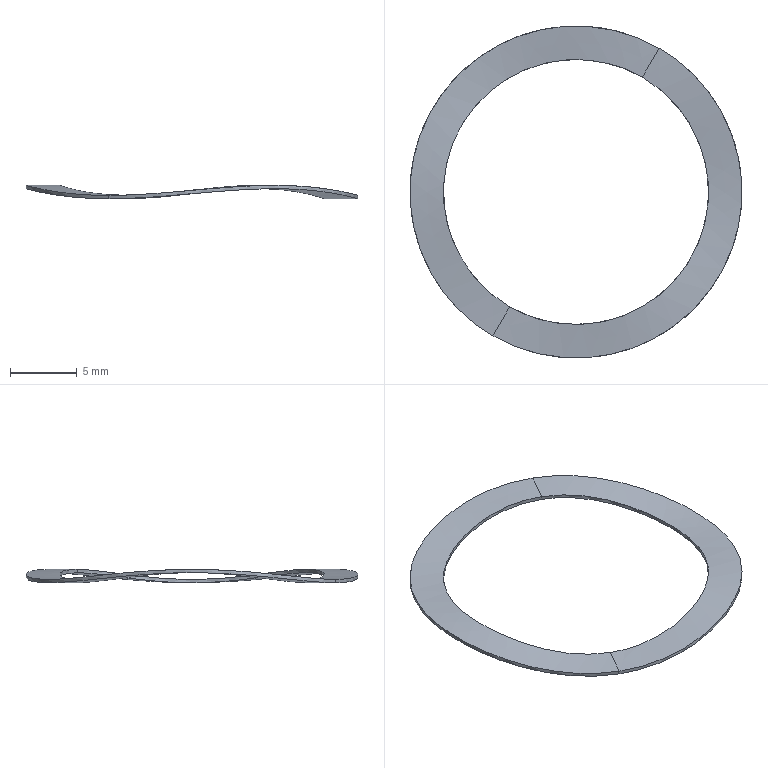Part | STEP file | TQ-DD-1105-THWWasher1010_デフォルト | 1 solid | 8 faces | box 24.801 x 24.797 x 1.007 mm | volume 43.898 mm3 | spline 8
STEP:
#1=CARTESIAN_POINT('',(6.2,10.738,1.));
#2=VERTEX_POINT('',#1);
#3=CARTESIAN_POINT('',(-6.201,-10.74,0.25));
#4=VERTEX_POINT('',#3);
#5=CARTESIAN_POINT('',(6.2,10.738,1.));
#6=CARTESIAN_POINT('',(4.132,11.932,1.));
#7=CARTESIAN_POINT('',(1.777,12.627,0.8423));
#8=CARTESIAN_POINT('',(-0.6996,12.727,0.5274));
#9=CARTESIAN_POINT('',(-4.616,11.93,0.187));
#10=CARTESIAN_POINT('',(-7.888,9.748,0.2524));
#11=CARTESIAN_POINT('',(-9.016,8.711,0.3521));
#12=CARTESIAN_POINT('',(-10.994,6.248,0.6338));
#13=CARTESIAN_POINT('',(-12.127,3.276,0.917));
#14=CARTESIAN_POINT('',(-12.457,1.647,1.018));
#15=CARTESIAN_POINT('',(-12.579,-2.323,1.042));
#16=CARTESIAN_POINT('',(-11.175,-6.066,0.6803));
#17=CARTESIAN_POINT('',(-9.869,-8.021,0.3939));
#18=CARTESIAN_POINT('',(-8.165,-9.606,0.25));
#19=CARTESIAN_POINT('',(-6.201,-10.74,0.25));
#20=B_SPLINE_CURVE_WITH_KNOTS('',5,(#5,#6,#7,#8,#9,#10,#11,#12,#13,#14,#15,#16,#17,#18,#19),.UNSPECIFIED.,.F.,.F.,(6,3,3,3,6),(0.,10.77,17.632,25.007,35.289),.UNSPECIFIED.);
#21=EDGE_CURVE('',#2,#4,#20,.T.);
#22=ORIENTED_EDGE('',*,*,#21,.T.);
#23=CARTESIAN_POINT('',(-4.951,-8.575,0.2603));
#24=VERTEX_POINT('',#23);
#25=CARTESIAN_POINT('',(-5.576,-9.657,0.2552));
#26=DIRECTION('',(0.5,0.866,0.004128));
#27=VECTOR('',#26,1000.);
#28=LINE('',#25,#27);
#29=EDGE_CURVE('',#4,#24,#28,.T.);
#30=ORIENTED_EDGE('',*,*,#29,.T.);
#31=CARTESIAN_POINT('',(4.95,8.573,0.9966));
#32=VERTEX_POINT('',#31);
#33=CARTESIAN_POINT('',(-4.951,-8.575,0.2603));
#34=CARTESIAN_POINT('',(-6.515,-7.671,0.2603));
#35=CARTESIAN_POINT('',(-7.873,-6.41,0.4039));
#36=CARTESIAN_POINT('',(-8.92,-4.849,0.6897));
#37=CARTESIAN_POINT('',(-10.044,-1.857,1.05));
#38=CARTESIAN_POINT('',(-9.946,1.316,1.024));
#39=CARTESIAN_POINT('',(-9.681,2.618,0.9223));
#40=CARTESIAN_POINT('',(-8.774,4.993,0.6373));
#41=CARTESIAN_POINT('',(-7.195,6.959,0.3538));
#42=CARTESIAN_POINT('',(-6.295,7.784,0.2533));
#43=CARTESIAN_POINT('',(-3.689,9.522,0.1859));
#44=CARTESIAN_POINT('',(-0.5659,10.16,0.5249));
#45=CARTESIAN_POINT('',(1.416,10.081,0.8392));
#46=CARTESIAN_POINT('',(3.298,9.527,0.9966));
#47=CARTESIAN_POINT('',(4.95,8.573,0.9966));
#48=B_SPLINE_CURVE_WITH_KNOTS('',5,(#33,#34,#35,#36,#37,#38,#39,#40,#41,#42,#43,#44,#45,#46,#47),.UNSPECIFIED.,.F.,.F.,(6,3,3,3,6),(0.,10.282,17.658,24.519,35.289),.UNSPECIFIED.);
#49=EDGE_CURVE('',#24,#32,#48,.T.);
#50=ORIENTED_EDGE('',*,*,#49,.T.);
#51=CARTESIAN_POINT('',(5.575,9.656,0.9983));
#52=DIRECTION('',(0.5,0.866,0.001376));
#53=VECTOR('',#52,1000.);
#54=LINE('',#51,#53);
#55=EDGE_CURVE('',#32,#2,#54,.T.);
#56=ORIENTED_EDGE('',*,*,#55,.T.);
#57=EDGE_LOOP('',(#22,#30,#50,#56));
#58=FACE_OUTER_BOUND('',#57,.T.);
#59=CARTESIAN_POINT('',(6.2,10.738,1.));
#60=CARTESIAN_POINT('',(4.95,8.573,0.9966));
#61=CARTESIAN_POINT('',(4.132,11.932,1.));
#62=CARTESIAN_POINT('',(3.298,9.527,0.9966));
#63=CARTESIAN_POINT('',(1.777,12.627,0.8423));
#64=CARTESIAN_POINT('',(1.416,10.081,0.8392));
#65=CARTESIAN_POINT('',(-0.6996,12.727,0.5274));
#66=CARTESIAN_POINT('',(-0.5659,10.16,0.5249));
#67=CARTESIAN_POINT('',(-4.616,11.93,0.187));
#68=CARTESIAN_POINT('',(-3.689,9.522,0.1859));
#69=CARTESIAN_POINT('',(-7.888,9.748,0.2524));
#70=CARTESIAN_POINT('',(-6.295,7.784,0.2533));
#71=CARTESIAN_POINT('',(-9.016,8.711,0.3521));
#72=CARTESIAN_POINT('',(-7.195,6.959,0.3538));
#73=CARTESIAN_POINT('',(-10.994,6.248,0.6338));
#74=CARTESIAN_POINT('',(-8.774,4.993,0.6373));
#75=CARTESIAN_POINT('',(-12.127,3.276,0.917));
#76=CARTESIAN_POINT('',(-9.681,2.618,0.9223));
#77=CARTESIAN_POINT('',(-12.457,1.647,1.018));
#78=CARTESIAN_POINT('',(-9.946,1.316,1.024));
#79=CARTESIAN_POINT('',(-12.579,-2.323,1.042));
#80=CARTESIAN_POINT('',(-10.044,-1.857,1.05));
#81=CARTESIAN_POINT('',(-11.175,-6.066,0.6803));
#82=CARTESIAN_POINT('',(-8.92,-4.849,0.6897));
#83=CARTESIAN_POINT('',(-9.869,-8.021,0.3939));
#84=CARTESIAN_POINT('',(-7.873,-6.41,0.4039));
#85=CARTESIAN_POINT('',(-8.165,-9.606,0.25));
#86=CARTESIAN_POINT('',(-6.515,-7.671,0.2603));
#87=CARTESIAN_POINT('',(-6.201,-10.74,0.25));
#88=CARTESIAN_POINT('',(-4.951,-8.575,0.2603));
#89=B_SPLINE_SURFACE_WITH_KNOTS('',5,1,((#59,#60),(#61,#62),(#63,#64),(#65,#66),(#67,#68),(#69,#70),(#71,#72),(#73,#74),(#75,#76),(#77,#78),(#79,#80),(#81,#82),(#83,#84),(#85,#86),(#87,#88)),.UNSPECIFIED.,.F.,.F.,.F.,(6,3,3,3,6),(2,2),(0.,10.77,17.632,25.007,35.289),(-12.4,-9.9),.UNSPECIFIED.);
#90=ADVANCED_FACE('',(#58),#89,.T.);
#91=CARTESIAN_POINT('',(-6.201,-10.74,0.25));
#92=CARTESIAN_POINT('',(-4.236,-11.874,0.25));
#93=CARTESIAN_POINT('',(-2.012,-12.557,0.3939));
#94=CARTESIAN_POINT('',(0.334,-12.711,0.6803));
#95=CARTESIAN_POINT('',(4.199,-12.069,1.035));
#96=CARTESIAN_POINT('',(7.52,-10.047,1.019));
#97=CARTESIAN_POINT('',(8.722,-9.019,0.9309));
#98=CARTESIAN_POINT('',(10.785,-6.602,0.6607));
#99=CARTESIAN_POINT('',(11.999,-3.682,0.3679));
#100=CARTESIAN_POINT('',(12.376,-2.114,0.2551));
#101=CARTESIAN_POINT('',(12.665,1.892,0.1802));
#102=CARTESIAN_POINT('',(11.372,5.758,0.5274));
#103=CARTESIAN_POINT('',(10.047,7.852,0.8423));
#104=CARTESIAN_POINT('',(8.267,9.545,1.));
#105=CARTESIAN_POINT('',(6.2,10.738,1.));
#106=B_SPLINE_CURVE_WITH_KNOTS('',5,(#91,#92,#93,#94,#95,#96,#97,#98,#99,#100,#101,#102,#103,#104,#105),.UNSPECIFIED.,.F.,.F.,(6,3,3,3,6),(0.,10.282,17.307,24.519,35.29),.UNSPECIFIED.);
#107=EDGE_CURVE('',#4,#2,#106,.T.);
#108=ORIENTED_EDGE('',*,*,#107,.T.);
#109=ORIENTED_EDGE('',*,*,#55,.F.);
#110=CARTESIAN_POINT('',(4.95,8.573,0.9966));
#111=CARTESIAN_POINT('',(6.601,7.62,0.9966));
#112=CARTESIAN_POINT('',(8.023,6.267,0.8392));
#113=CARTESIAN_POINT('',(9.082,4.59,0.5249));
#114=CARTESIAN_POINT('',(10.111,1.506,0.1792));
#115=CARTESIAN_POINT('',(9.88,-1.684,0.2562));
#116=CARTESIAN_POINT('',(9.582,-2.934,0.3698));
#117=CARTESIAN_POINT('',(8.613,-5.266,0.6643));
#118=CARTESIAN_POINT('',(6.965,-7.199,0.9362));
#119=CARTESIAN_POINT('',(6.005,-8.021,1.025));
#120=CARTESIAN_POINT('',(3.352,-9.637,1.043));
#121=CARTESIAN_POINT('',(0.261,-10.149,0.6897));
#122=CARTESIAN_POINT('',(-1.615,-10.023,0.4039));
#123=CARTESIAN_POINT('',(-3.386,-9.478,0.2603));
#124=CARTESIAN_POINT('',(-4.951,-8.575,0.2603));
#125=B_SPLINE_CURVE_WITH_KNOTS('',5,(#110,#111,#112,#113,#114,#115,#116,#117,#118,#119,#120,#121,#122,#123,#124),.UNSPECIFIED.,.F.,.F.,(6,3,3,3,6),(0.,10.771,17.982,25.008,35.29),.UNSPECIFIED.);
#126=EDGE_CURVE('',#32,#24,#125,.T.);
#127=ORIENTED_EDGE('',*,*,#126,.T.);
#128=ORIENTED_EDGE('',*,*,#29,.F.);
#129=EDGE_LOOP('',(#108,#109,#127,#128));
#130=FACE_OUTER_BOUND('',#129,.T.);
#131=CARTESIAN_POINT('',(-6.201,-10.74,0.25));
#132=CARTESIAN_POINT('',(-4.951,-8.575,0.2603));
#133=CARTESIAN_POINT('',(-4.236,-11.874,0.25));
#134=CARTESIAN_POINT('',(-3.386,-9.478,0.2603));
#135=CARTESIAN_POINT('',(-2.012,-12.557,0.3939));
#136=CARTESIAN_POINT('',(-1.615,-10.023,0.4039));
#137=CARTESIAN_POINT('',(0.334,-12.711,0.6803));
#138=CARTESIAN_POINT('',(0.261,-10.149,0.6897));
#139=CARTESIAN_POINT('',(4.199,-12.069,1.035));
#140=CARTESIAN_POINT('',(3.352,-9.637,1.043));
#141=CARTESIAN_POINT('',(7.52,-10.047,1.019));
#142=CARTESIAN_POINT('',(6.005,-8.021,1.025));
#143=CARTESIAN_POINT('',(8.722,-9.019,0.9309));
#144=CARTESIAN_POINT('',(6.965,-7.199,0.9362));
#145=CARTESIAN_POINT('',(10.785,-6.602,0.6607));
#146=CARTESIAN_POINT('',(8.613,-5.266,0.6643));
#147=CARTESIAN_POINT('',(11.999,-3.682,0.3679));
#148=CARTESIAN_POINT('',(9.582,-2.934,0.3698));
#149=CARTESIAN_POINT('',(12.376,-2.114,0.2551));
#150=CARTESIAN_POINT('',(9.88,-1.684,0.2562));
#151=CARTESIAN_POINT('',(12.665,1.892,0.1802));
#152=CARTESIAN_POINT('',(10.111,1.506,0.1792));
#153=CARTESIAN_POINT('',(11.372,5.758,0.5274));
#154=CARTESIAN_POINT('',(9.082,4.59,0.5249));
#155=CARTESIAN_POINT('',(10.047,7.852,0.8423));
#156=CARTESIAN_POINT('',(8.023,6.267,0.8392));
#157=CARTESIAN_POINT('',(8.267,9.545,1.));
#158=CARTESIAN_POINT('',(6.601,7.62,0.9966));
#159=CARTESIAN_POINT('',(6.2,10.738,1.));
#160=CARTESIAN_POINT('',(4.95,8.573,0.9966));
#161=B_SPLINE_SURFACE_WITH_KNOTS('',5,1,((#131,#132),(#133,#134),(#135,#136),(#137,#138),(#139,#140),(#141,#142),(#143,#144),(#145,#146),(#147,#148),(#149,#150),(#151,#152),(#153,#154),(#155,#156),(#157,#158),(#159,#160)),.UNSPECIFIED.,.F.,.F.,.F.,(6,3,3,3,6),(2,2),(0.,10.282,17.307,24.519,35.29),(-12.4,-9.9),.UNSPECIFIED.);
#162=ADVANCED_FACE('',(#130),#161,.T.);
#163=CARTESIAN_POINT('',(6.2,10.739,0.75));
#164=VERTEX_POINT('',#163);
#165=CARTESIAN_POINT('',(6.2,10.739,0.875));
#166=DIRECTION('',(-0.000688,-0.001192,1.));
#167=VECTOR('',#166,1000.);
#168=LINE('',#165,#167);
#169=EDGE_CURVE('',#164,#2,#168,.T.);
#170=ORIENTED_EDGE('',*,*,#169,.F.);
#171=CARTESIAN_POINT('',(-6.2,-10.739,0.));
#172=VERTEX_POINT('',#171);
#173=CARTESIAN_POINT('',(-6.2,-10.739,0.));
#174=CARTESIAN_POINT('',(-8.175,-9.598,0.));
#175=CARTESIAN_POINT('',(-9.887,-8.003,0.1447));
#176=CARTESIAN_POINT('',(-11.187,-6.04,0.4318));
#177=CARTESIAN_POINT('',(-12.577,-2.308,0.7919));
#178=CARTESIAN_POINT('',(-12.455,1.637,0.7681));
#179=CARTESIAN_POINT('',(-12.13,3.258,0.6677));
#180=CARTESIAN_POINT('',(-11.007,6.224,0.3852));
#181=CARTESIAN_POINT('',(-9.03,8.698,0.1027));
#182=CARTESIAN_POINT('',(-7.898,9.742,0.002344));
#183=CARTESIAN_POINT('',(-4.606,11.938,-0.06333));
#184=CARTESIAN_POINT('',(-0.6705,12.732,0.2788));
#185=CARTESIAN_POINT('',(1.803,12.619,0.5932));
#186=CARTESIAN_POINT('',(4.144,11.926,0.75));
#187=CARTESIAN_POINT('',(6.2,10.739,0.75));
#188=B_SPLINE_CURVE_WITH_KNOTS('',5,(#173,#174,#175,#176,#177,#178,#179,#180,#181,#182,#183,#184,#185,#186,#187),.UNSPECIFIED.,.F.,.F.,(6,3,3,3,6),(0.,10.282,17.658,24.519,35.289),.UNSPECIFIED.);
#189=EDGE_CURVE('',#172,#164,#188,.T.);
#190=ORIENTED_EDGE('',*,*,#189,.F.);
#191=CARTESIAN_POINT('',(-6.2,-10.739,0.125));
#192=DIRECTION('',(0.002064,0.003575,-1.));
#193=VECTOR('',#192,1000.);
#194=LINE('',#191,#193);
#195=EDGE_CURVE('',#4,#172,#194,.T.);
#196=ORIENTED_EDGE('',*,*,#195,.F.);
#197=ORIENTED_EDGE('',*,*,#21,.F.);
#198=EDGE_LOOP('',(#170,#190,#196,#197));
#199=FACE_OUTER_BOUND('',#198,.T.);
#200=CARTESIAN_POINT('',(6.2,10.738,1.));
#201=CARTESIAN_POINT('',(6.2,10.739,0.75));
#202=CARTESIAN_POINT('',(4.132,11.932,1.));
#203=CARTESIAN_POINT('',(4.144,11.926,0.75));
#204=CARTESIAN_POINT('',(1.777,12.627,0.8423));
#205=CARTESIAN_POINT('',(1.803,12.619,0.5932));
#206=CARTESIAN_POINT('',(-0.6996,12.727,0.5274));
#207=CARTESIAN_POINT('',(-0.6705,12.732,0.2788));
#208=CARTESIAN_POINT('',(-4.616,11.93,0.187));
#209=CARTESIAN_POINT('',(-4.606,11.938,-0.06333));
#210=CARTESIAN_POINT('',(-7.888,9.748,0.2524));
#211=CARTESIAN_POINT('',(-7.898,9.742,0.002344));
#212=CARTESIAN_POINT('',(-9.016,8.711,0.3521));
#213=CARTESIAN_POINT('',(-9.03,8.698,0.1027));
#214=CARTESIAN_POINT('',(-10.994,6.248,0.6338));
#215=CARTESIAN_POINT('',(-11.007,6.224,0.3852));
#216=CARTESIAN_POINT('',(-12.127,3.276,0.917));
#217=CARTESIAN_POINT('',(-12.13,3.258,0.6677));
#218=CARTESIAN_POINT('',(-12.457,1.647,1.018));
#219=CARTESIAN_POINT('',(-12.455,1.637,0.7681));
#220=CARTESIAN_POINT('',(-12.579,-2.323,1.042));
#221=CARTESIAN_POINT('',(-12.577,-2.308,0.7919));
#222=CARTESIAN_POINT('',(-11.175,-6.066,0.6803));
#223=CARTESIAN_POINT('',(-11.187,-6.04,0.4318));
#224=CARTESIAN_POINT('',(-9.869,-8.021,0.3939));
#225=CARTESIAN_POINT('',(-9.887,-8.003,0.1447));
#226=CARTESIAN_POINT('',(-8.165,-9.606,0.25));
#227=CARTESIAN_POINT('',(-8.175,-9.598,0.));
#228=CARTESIAN_POINT('',(-6.201,-10.74,0.25));
#229=CARTESIAN_POINT('',(-6.2,-10.739,0.));
#230=B_SPLINE_SURFACE_WITH_KNOTS('',5,1,((#200,#201),(#202,#203),(#204,#205),(#206,#207),(#208,#209),(#210,#211),(#212,#213),(#214,#215),(#216,#217),(#218,#219),(#220,#221),(#222,#223),(#224,#225),(#226,#227),(#228,#229)),.UNSPECIFIED.,.F.,.F.,.F.,(6,3,3,3,6),(2,2),(0.,10.77,17.632,25.007,35.289),(-0.125,0.125),.UNSPECIFIED.);
#231=ADVANCED_FACE('',(#199),#230,.F.);
#232=CARTESIAN_POINT('',(4.95,8.574,0.7466));
#233=VERTEX_POINT('',#232);
#234=CARTESIAN_POINT('',(4.95,8.574,0.8716));
#235=DIRECTION('',(0.000688,0.001192,-1.));
#236=VECTOR('',#235,1000.);
#237=LINE('',#234,#236);
#238=EDGE_CURVE('',#32,#233,#237,.T.);
#239=ORIENTED_EDGE('',*,*,#238,.F.);
#240=ORIENTED_EDGE('',*,*,#49,.F.);
#241=CARTESIAN_POINT('',(-4.95,-8.574,0.01032));
#242=VERTEX_POINT('',#241);
#243=CARTESIAN_POINT('',(-4.95,-8.574,0.1353));
#244=DIRECTION('',(-0.002064,-0.003575,1.));
#245=VECTOR('',#244,1000.);
#246=LINE('',#243,#245);
#247=EDGE_CURVE('',#242,#24,#246,.T.);
#248=ORIENTED_EDGE('',*,*,#247,.F.);
#249=CARTESIAN_POINT('',(4.95,8.574,0.7466));
#250=CARTESIAN_POINT('',(3.31,9.521,0.7466));
#251=CARTESIAN_POINT('',(1.442,10.074,0.5901));
#252=CARTESIAN_POINT('',(-0.5367,10.164,0.2763));
#253=CARTESIAN_POINT('',(-3.679,9.531,-0.06435));
#254=CARTESIAN_POINT('',(-6.305,7.779,0.003297));
#255=CARTESIAN_POINT('',(-7.208,6.945,0.1045));
#256=CARTESIAN_POINT('',(-8.787,4.969,0.3887));
#257=CARTESIAN_POINT('',(-9.685,2.6,0.6729));
#258=CARTESIAN_POINT('',(-9.944,1.306,0.7743));
#259=CARTESIAN_POINT('',(-10.042,-1.841,0.8));
#260=CARTESIAN_POINT('',(-8.931,-4.822,0.4412));
#261=CARTESIAN_POINT('',(-7.891,-6.392,0.1547));
#262=CARTESIAN_POINT('',(-6.525,-7.664,0.01032));
#263=CARTESIAN_POINT('',(-4.95,-8.574,0.01032));
#264=B_SPLINE_CURVE_WITH_KNOTS('',5,(#249,#250,#251,#252,#253,#254,#255,#256,#257,#258,#259,#260,#261,#262,#263),.UNSPECIFIED.,.F.,.F.,(6,3,3,3,6),(0.,10.77,17.632,25.007,35.289),.UNSPECIFIED.);
#265=EDGE_CURVE('',#233,#242,#264,.T.);
#266=ORIENTED_EDGE('',*,*,#265,.F.);
#267=EDGE_LOOP('',(#239,#240,#248,#266));
#268=FACE_OUTER_BOUND('',#267,.T.);
#269=CARTESIAN_POINT('',(4.95,8.574,0.7466));
#270=CARTESIAN_POINT('',(4.95,8.573,0.9966));
#271=CARTESIAN_POINT('',(3.31,9.521,0.7466));
#272=CARTESIAN_POINT('',(3.298,9.527,0.9966));
#273=CARTESIAN_POINT('',(1.442,10.074,0.5901));
#274=CARTESIAN_POINT('',(1.416,10.081,0.8392));
#275=CARTESIAN_POINT('',(-0.5367,10.164,0.2763));
#276=CARTESIAN_POINT('',(-0.5659,10.16,0.5249));
#277=CARTESIAN_POINT('',(-3.679,9.531,-0.06435));
#278=CARTESIAN_POINT('',(-3.689,9.522,0.1859));
#279=CARTESIAN_POINT('',(-6.305,7.779,0.003297));
#280=CARTESIAN_POINT('',(-6.295,7.784,0.2533));
#281=CARTESIAN_POINT('',(-7.208,6.945,0.1045));
#282=CARTESIAN_POINT('',(-7.195,6.959,0.3538));
#283=CARTESIAN_POINT('',(-8.787,4.969,0.3887));
#284=CARTESIAN_POINT('',(-8.774,4.993,0.6373));
#285=CARTESIAN_POINT('',(-9.685,2.6,0.6729));
#286=CARTESIAN_POINT('',(-9.681,2.618,0.9223));
#287=CARTESIAN_POINT('',(-9.944,1.306,0.7743));
#288=CARTESIAN_POINT('',(-9.946,1.316,1.024));
#289=CARTESIAN_POINT('',(-10.042,-1.841,0.8));
#290=CARTESIAN_POINT('',(-10.044,-1.857,1.05));
#291=CARTESIAN_POINT('',(-8.931,-4.822,0.4412));
#292=CARTESIAN_POINT('',(-8.92,-4.849,0.6897));
#293=CARTESIAN_POINT('',(-7.891,-6.392,0.1547));
#294=CARTESIAN_POINT('',(-7.873,-6.41,0.4039));
#295=CARTESIAN_POINT('',(-6.525,-7.664,0.01032));
#296=CARTESIAN_POINT('',(-6.515,-7.671,0.2603));
#297=CARTESIAN_POINT('',(-4.95,-8.574,0.01032));
#298=CARTESIAN_POINT('',(-4.951,-8.575,0.2603));
#299=B_SPLINE_SURFACE_WITH_KNOTS('',5,1,((#269,#270),(#271,#272),(#273,#274),(#275,#276),(#277,#278),(#279,#280),(#281,#282),(#283,#284),(#285,#286),(#287,#288),(#289,#290),(#291,#292),(#293,#294),(#295,#296),(#297,#298)),.UNSPECIFIED.,.F.,.F.,.F.,(6,3,3,3,6),(2,2),(0.,10.77,17.632,25.007,35.289),(0.,0.25),.UNSPECIFIED.);
#300=ADVANCED_FACE('',(#268),#299,.F.);
#301=ORIENTED_EDGE('',*,*,#195,.T.);
#302=CARTESIAN_POINT('',(6.2,10.739,0.75));
#303=CARTESIAN_POINT('',(8.256,9.552,0.75));
#304=CARTESIAN_POINT('',(10.027,7.871,0.5932));
#305=CARTESIAN_POINT('',(11.361,5.785,0.2788));
#306=CARTESIAN_POINT('',(12.667,1.905,-0.07013));
#307=CARTESIAN_POINT('',(12.375,-2.126,0.005117));
#308=CARTESIAN_POINT('',(11.994,-3.702,0.1187));
#309=CARTESIAN_POINT('',(10.77,-6.624,0.4121));
#310=CARTESIAN_POINT('',(8.708,-9.03,0.6814));
#311=CARTESIAN_POINT('',(7.512,-10.05,0.7689));
#312=CARTESIAN_POINT('',(4.212,-12.059,0.7848));
#313=CARTESIAN_POINT('',(0.3628,-12.708,0.4317));
#314=CARTESIAN_POINT('',(-1.987,-12.564,0.1447));
#315=CARTESIAN_POINT('',(-4.225,-11.879,0.));
#316=CARTESIAN_POINT('',(-6.2,-10.739,0.));
#317=B_SPLINE_CURVE_WITH_KNOTS('',5,(#302,#303,#304,#305,#306,#307,#308,#309,#310,#311,#312,#313,#314,#315,#316),.UNSPECIFIED.,.F.,.F.,(6,3,3,3,6),(0.,10.771,17.982,25.008,35.29),.UNSPECIFIED.);
#318=EDGE_CURVE('',#164,#172,#317,.T.);
#319=ORIENTED_EDGE('',*,*,#318,.F.);
#320=ORIENTED_EDGE('',*,*,#169,.T.);
#321=ORIENTED_EDGE('',*,*,#107,.F.);
#322=EDGE_LOOP('',(#301,#319,#320,#321));
#323=FACE_OUTER_BOUND('',#322,.T.);
#324=CARTESIAN_POINT('',(-6.201,-10.74,0.25));
#325=CARTESIAN_POINT('',(-6.2,-10.739,0.));
#326=CARTESIAN_POINT('',(-4.236,-11.874,0.25));
#327=CARTESIAN_POINT('',(-4.225,-11.879,0.));
#328=CARTESIAN_POINT('',(-2.012,-12.557,0.3939));
#329=CARTESIAN_POINT('',(-1.987,-12.564,0.1447));
#330=CARTESIAN_POINT('',(0.334,-12.711,0.6803));
#331=CARTESIAN_POINT('',(0.3628,-12.708,0.4317));
#332=CARTESIAN_POINT('',(4.199,-12.069,1.035));
#333=CARTESIAN_POINT('',(4.212,-12.059,0.7848));
#334=CARTESIAN_POINT('',(7.52,-10.047,1.019));
#335=CARTESIAN_POINT('',(7.512,-10.05,0.7689));
#336=CARTESIAN_POINT('',(8.722,-9.019,0.9309));
#337=CARTESIAN_POINT('',(8.708,-9.03,0.6814));
#338=CARTESIAN_POINT('',(10.785,-6.602,0.6607));
#339=CARTESIAN_POINT('',(10.77,-6.624,0.4121));
#340=CARTESIAN_POINT('',(11.999,-3.682,0.3679));
#341=CARTESIAN_POINT('',(11.994,-3.702,0.1187));
#342=CARTESIAN_POINT('',(12.376,-2.114,0.2551));
#343=CARTESIAN_POINT('',(12.375,-2.126,0.005117));
#344=CARTESIAN_POINT('',(12.665,1.892,0.1802));
#345=CARTESIAN_POINT('',(12.667,1.905,-0.07013));
#346=CARTESIAN_POINT('',(11.372,5.758,0.5274));
#347=CARTESIAN_POINT('',(11.361,5.785,0.2788));
#348=CARTESIAN_POINT('',(10.047,7.852,0.8423));
#349=CARTESIAN_POINT('',(10.027,7.871,0.5932));
#350=CARTESIAN_POINT('',(8.267,9.545,1.));
#351=CARTESIAN_POINT('',(8.256,9.552,0.75));
#352=CARTESIAN_POINT('',(6.2,10.738,1.));
#353=CARTESIAN_POINT('',(6.2,10.739,0.75));
#354=B_SPLINE_SURFACE_WITH_KNOTS('',5,1,((#324,#325),(#326,#327),(#328,#329),(#330,#331),(#332,#333),(#334,#335),(#336,#337),(#338,#339),(#340,#341),(#342,#343),(#344,#345),(#346,#347),(#348,#349),(#350,#351),(#352,#353)),.UNSPECIFIED.,.F.,.F.,.F.,(6,3,3,3,6),(2,2),(0.,10.282,17.307,24.519,35.29),(-0.125,0.125),.UNSPECIFIED.);
#355=ADVANCED_FACE('',(#323),#354,.F.);
#356=ORIENTED_EDGE('',*,*,#247,.T.);
#357=ORIENTED_EDGE('',*,*,#126,.F.);
#358=ORIENTED_EDGE('',*,*,#238,.T.);
#359=CARTESIAN_POINT('',(-4.95,-8.574,0.01032));
#360=CARTESIAN_POINT('',(-3.375,-9.483,0.01032));
#361=CARTESIAN_POINT('',(-1.59,-10.03,0.1547));
#362=CARTESIAN_POINT('',(0.2897,-10.145,0.4412));
#363=CARTESIAN_POINT('',(3.364,-9.627,0.7928));
#364=CARTESIAN_POINT('',(5.997,-8.024,0.7751));
#365=CARTESIAN_POINT('',(6.952,-7.21,0.6868));
#366=CARTESIAN_POINT('',(8.599,-5.289,0.4157));
#367=CARTESIAN_POINT('',(9.576,-2.954,0.1206));
#368=CARTESIAN_POINT('',(9.88,-1.696,0.006149));
#369=CARTESIAN_POINT('',(10.113,1.519,-0.07112));
#370=CARTESIAN_POINT('',(9.071,4.617,0.2763));
#371=CARTESIAN_POINT('',(8.003,6.286,0.5901));
#372=CARTESIAN_POINT('',(6.59,7.627,0.7466));
#373=CARTESIAN_POINT('',(4.95,8.574,0.7466));
#374=B_SPLINE_CURVE_WITH_KNOTS('',5,(#359,#360,#361,#362,#363,#364,#365,#366,#367,#368,#369,#370,#371,#372,#373),.UNSPECIFIED.,.F.,.F.,(6,3,3,3,6),(0.,10.282,17.307,24.519,35.29),.UNSPECIFIED.);
#375=EDGE_CURVE('',#242,#233,#374,.T.);
#376=ORIENTED_EDGE('',*,*,#375,.F.);
#377=EDGE_LOOP('',(#356,#357,#358,#376));
#378=FACE_OUTER_BOUND('',#377,.T.);
#379=CARTESIAN_POINT('',(-4.95,-8.574,0.01032));
#380=CARTESIAN_POINT('',(-4.951,-8.575,0.2603));
#381=CARTESIAN_POINT('',(-3.375,-9.483,0.01032));
#382=CARTESIAN_POINT('',(-3.386,-9.478,0.2603));
#383=CARTESIAN_POINT('',(-1.59,-10.03,0.1547));
#384=CARTESIAN_POINT('',(-1.615,-10.023,0.4039));
#385=CARTESIAN_POINT('',(0.2897,-10.145,0.4412));
#386=CARTESIAN_POINT('',(0.261,-10.149,0.6897));
#387=CARTESIAN_POINT('',(3.364,-9.627,0.7928));
#388=CARTESIAN_POINT('',(3.352,-9.637,1.043));
#389=CARTESIAN_POINT('',(5.997,-8.024,0.7751));
#390=CARTESIAN_POINT('',(6.005,-8.021,1.025));
#391=CARTESIAN_POINT('',(6.952,-7.21,0.6868));
#392=CARTESIAN_POINT('',(6.965,-7.199,0.9362));
#393=CARTESIAN_POINT('',(8.599,-5.289,0.4157));
#394=CARTESIAN_POINT('',(8.613,-5.266,0.6643));
#395=CARTESIAN_POINT('',(9.576,-2.954,0.1206));
#396=CARTESIAN_POINT('',(9.582,-2.934,0.3698));
#397=CARTESIAN_POINT('',(9.88,-1.696,0.006149));
#398=CARTESIAN_POINT('',(9.88,-1.684,0.2562));
#399=CARTESIAN_POINT('',(10.113,1.519,-0.07112));
#400=CARTESIAN_POINT('',(10.111,1.506,0.1792));
#401=CARTESIAN_POINT('',(9.071,4.617,0.2763));
#402=CARTESIAN_POINT('',(9.082,4.59,0.5249));
#403=CARTESIAN_POINT('',(8.003,6.286,0.5901));
#404=CARTESIAN_POINT('',(8.023,6.267,0.8392));
#405=CARTESIAN_POINT('',(6.59,7.627,0.7466));
#406=CARTESIAN_POINT('',(6.601,7.62,0.9966));
#407=CARTESIAN_POINT('',(4.95,8.574,0.7466));
#408=CARTESIAN_POINT('',(4.95,8.573,0.9966));
#409=B_SPLINE_SURFACE_WITH_KNOTS('',5,1,((#379,#380),(#381,#382),(#383,#384),(#385,#386),(#387,#388),(#389,#390),(#391,#392),(#393,#394),(#395,#396),(#397,#398),(#399,#400),(#401,#402),(#403,#404),(#405,#406),(#407,#408)),.UNSPECIFIED.,.F.,.F.,.F.,(6,3,3,3,6),(2,2),(0.,10.282,17.307,24.519,35.29),(0.,0.25),.UNSPECIFIED.);
#410=ADVANCED_FACE('',(#378),#409,.F.);
#411=ORIENTED_EDGE('',*,*,#265,.T.);
#412=CARTESIAN_POINT('',(-5.575,-9.656,0.00516));
#413=DIRECTION('',(-0.5,-0.866,-0.004128));
#414=VECTOR('',#413,1000.);
#415=LINE('',#412,#414);
#416=EDGE_CURVE('',#242,#172,#415,.T.);
#417=ORIENTED_EDGE('',*,*,#416,.T.);
#418=ORIENTED_EDGE('',*,*,#189,.T.);
#419=CARTESIAN_POINT('',(5.575,9.656,0.7483));
#420=DIRECTION('',(-0.5,-0.866,-0.001376));
#421=VECTOR('',#420,1000.);
#422=LINE('',#419,#421);
#423=EDGE_CURVE('',#164,#233,#422,.T.);
#424=ORIENTED_EDGE('',*,*,#423,.T.);
#425=EDGE_LOOP('',(#411,#417,#418,#424));
#426=FACE_OUTER_BOUND('',#425,.T.);
#427=CARTESIAN_POINT('',(4.95,8.574,0.7466));
#428=CARTESIAN_POINT('',(6.2,10.739,0.75));
#429=CARTESIAN_POINT('',(3.31,9.521,0.7466));
#430=CARTESIAN_POINT('',(4.144,11.926,0.75));
#431=CARTESIAN_POINT('',(1.442,10.074,0.5901));
#432=CARTESIAN_POINT('',(1.803,12.619,0.5932));
#433=CARTESIAN_POINT('',(-0.5367,10.164,0.2763));
#434=CARTESIAN_POINT('',(-0.6705,12.732,0.2788));
#435=CARTESIAN_POINT('',(-3.679,9.531,-0.06435));
#436=CARTESIAN_POINT('',(-4.606,11.938,-0.06333));
#437=CARTESIAN_POINT('',(-6.305,7.779,0.003297));
#438=CARTESIAN_POINT('',(-7.898,9.742,0.002344));
#439=CARTESIAN_POINT('',(-7.208,6.945,0.1045));
#440=CARTESIAN_POINT('',(-9.03,8.698,0.1027));
#441=CARTESIAN_POINT('',(-8.787,4.969,0.3887));
#442=CARTESIAN_POINT('',(-11.007,6.224,0.3852));
#443=CARTESIAN_POINT('',(-9.685,2.6,0.6729));
#444=CARTESIAN_POINT('',(-12.13,3.258,0.6677));
#445=CARTESIAN_POINT('',(-9.944,1.306,0.7743));
#446=CARTESIAN_POINT('',(-12.455,1.637,0.7681));
#447=CARTESIAN_POINT('',(-10.042,-1.841,0.8));
#448=CARTESIAN_POINT('',(-12.577,-2.308,0.7919));
#449=CARTESIAN_POINT('',(-8.931,-4.822,0.4412));
#450=CARTESIAN_POINT('',(-11.187,-6.04,0.4318));
#451=CARTESIAN_POINT('',(-7.891,-6.392,0.1547));
#452=CARTESIAN_POINT('',(-9.887,-8.003,0.1447));
#453=CARTESIAN_POINT('',(-6.525,-7.664,0.01032));
#454=CARTESIAN_POINT('',(-8.175,-9.598,0.));
#455=CARTESIAN_POINT('',(-4.95,-8.574,0.01032));
#456=CARTESIAN_POINT('',(-6.2,-10.739,0.));
#457=B_SPLINE_SURFACE_WITH_KNOTS('',5,1,((#427,#428),(#429,#430),(#431,#432),(#433,#434),(#435,#436),(#437,#438),(#439,#440),(#441,#442),(#443,#444),(#445,#446),(#447,#448),(#449,#450),(#451,#452),(#453,#454),(#455,#456)),.UNSPECIFIED.,.F.,.F.,.F.,(6,3,3,3,6),(2,2),(0.,10.77,17.632,25.007,35.289),(-1.25,1.25),.UNSPECIFIED.);
#458=ADVANCED_FACE('',(#426),#457,.T.);
#459=ORIENTED_EDGE('',*,*,#375,.T.);
#460=ORIENTED_EDGE('',*,*,#423,.F.);
#461=ORIENTED_EDGE('',*,*,#318,.T.);
#462=ORIENTED_EDGE('',*,*,#416,.F.);
#463=EDGE_LOOP('',(#459,#460,#461,#462));
#464=FACE_OUTER_BOUND('',#463,.T.);
#465=CARTESIAN_POINT('',(-4.95,-8.574,0.01032));
#466=CARTESIAN_POINT('',(-6.2,-10.739,0.));
#467=CARTESIAN_POINT('',(-3.375,-9.483,0.01032));
#468=CARTESIAN_POINT('',(-4.225,-11.879,0.));
#469=CARTESIAN_POINT('',(-1.59,-10.03,0.1547));
#470=CARTESIAN_POINT('',(-1.987,-12.564,0.1447));
#471=CARTESIAN_POINT('',(0.2897,-10.145,0.4412));
#472=CARTESIAN_POINT('',(0.3628,-12.708,0.4317));
#473=CARTESIAN_POINT('',(3.364,-9.627,0.7928));
#474=CARTESIAN_POINT('',(4.212,-12.059,0.7848));
#475=CARTESIAN_POINT('',(5.997,-8.024,0.7751));
#476=CARTESIAN_POINT('',(7.512,-10.05,0.7689));
#477=CARTESIAN_POINT('',(6.952,-7.21,0.6868));
#478=CARTESIAN_POINT('',(8.708,-9.03,0.6814));
#479=CARTESIAN_POINT('',(8.599,-5.289,0.4157));
#480=CARTESIAN_POINT('',(10.77,-6.624,0.4121));
#481=CARTESIAN_POINT('',(9.576,-2.954,0.1206));
#482=CARTESIAN_POINT('',(11.994,-3.702,0.1187));
#483=CARTESIAN_POINT('',(9.88,-1.696,0.006149));
#484=CARTESIAN_POINT('',(12.375,-2.126,0.005117));
#485=CARTESIAN_POINT('',(10.113,1.519,-0.07112));
#486=CARTESIAN_POINT('',(12.667,1.905,-0.07013));
#487=CARTESIAN_POINT('',(9.071,4.617,0.2763));
#488=CARTESIAN_POINT('',(11.361,5.785,0.2788));
#489=CARTESIAN_POINT('',(8.003,6.286,0.5901));
#490=CARTESIAN_POINT('',(10.027,7.871,0.5932));
#491=CARTESIAN_POINT('',(6.59,7.627,0.7466));
#492=CARTESIAN_POINT('',(8.256,9.552,0.75));
#493=CARTESIAN_POINT('',(4.95,8.574,0.7466));
#494=CARTESIAN_POINT('',(6.2,10.739,0.75));
#495=B_SPLINE_SURFACE_WITH_KNOTS('',5,1,((#465,#466),(#467,#468),(#469,#470),(#471,#472),(#473,#474),(#475,#476),(#477,#478),(#479,#480),(#481,#482),(#483,#484),(#485,#486),(#487,#488),(#489,#490),(#491,#492),(#493,#494)),.UNSPECIFIED.,.F.,.F.,.F.,(6,3,3,3,6),(2,2),(0.,10.282,17.307,24.519,35.29),(-1.25,1.25),.UNSPECIFIED.);
#496=ADVANCED_FACE('',(#464),#495,.T.);
#497=CLOSED_SHELL('',(#90,#162,#231,#300,#355,#410,#458,#496));
#498=MANIFOLD_SOLID_BREP('',#497);
#499=CARTESIAN_POINT('',(0.,0.,0.));
#500=DIRECTION('',(0.,0.,1.));
#501=DIRECTION('',(1.,0.,0.));
#502=AXIS2_PLACEMENT_3D('',#499,#500,#501);
#503=(LENGTH_UNIT()NAMED_UNIT(*)SI_UNIT(.MILLI.,.METRE.));
#504=UNCERTAINTY_MEASURE_WITH_UNIT(LENGTH_MEASURE(0.00001),#503,'','');
#505=(NAMED_UNIT(*)PLANE_ANGLE_UNIT()SI_UNIT($,.RADIAN.));
#506=(NAMED_UNIT(*)SI_UNIT($,.STERADIAN.)SOLID_ANGLE_UNIT());
#507=(GEOMETRIC_REPRESENTATION_CONTEXT(3)GLOBAL_UNCERTAINTY_ASSIGNED_CONTEXT((#504))GLOBAL_UNIT_ASSIGNED_CONTEXT((#503,#505,#506))REPRESENTATION_CONTEXT('',''));
#508=ADVANCED_BREP_SHAPE_REPRESENTATION('',(#498,#502),#507);